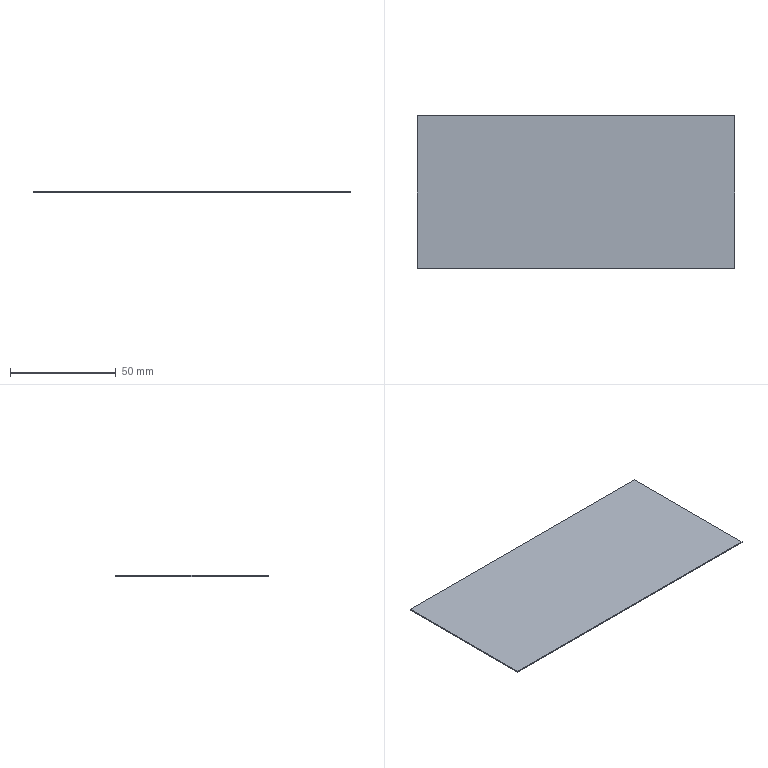Part | STEP file | Bag feed part 2 | 1 solid | 6 faces | box 150 x 72 x 0.5 mm | volume 5400 mm3 | plane 6
STEP:
#1=CARTESIAN_POINT('',(0.,0.,0.));
#2=DIRECTION('',(0.,0.,1.));
#3=DIRECTION('',(1.,0.,0.));
#4=AXIS2_PLACEMENT_3D('',#1,#2,#3);
#5=CARTESIAN_POINT('',(75.,-36.,0.));
#6=VERTEX_POINT('',#5);
#7=CARTESIAN_POINT('',(75.,36.,0.));
#8=VERTEX_POINT('',#7);
#9=CARTESIAN_POINT('',(75.,-36.,0.));
#10=DIRECTION('',(0.,1.,0.));
#11=VECTOR('',#10,1.);
#12=LINE('',#9,#11);
#13=CARTESIAN_POINT('',(75.,-36.,0.5));
#14=DIRECTION('',(-1.,0.,0.));
#15=DIRECTION('',(0.,0.,1.));
#16=AXIS2_PLACEMENT_3D('',#13,#14,#15);
#17=PLANE('',#16);
#18=CARTESIAN_POINT('',(-0.5,0.));
#19=DIRECTION('',(0.,1.));
#20=VECTOR('',#19,1.);
#21=LINE('',#18,#20);
#22=(GEOMETRIC_REPRESENTATION_CONTEXT(2)PARAMETRIC_REPRESENTATION_CONTEXT()REPRESENTATION_CONTEXT('',''));
#23=DEFINITIONAL_REPRESENTATION('',(#21),#22);
#24=PCURVE('',#17,#23);
#25=CARTESIAN_POINT('',(0.,0.,0.));
#26=DIRECTION('',(0.,0.,-1.));
#27=DIRECTION('',(-1.,0.,0.));
#28=AXIS2_PLACEMENT_3D('',#25,#26,#27);
#29=PLANE('',#28);
#30=CARTESIAN_POINT('',(-75.,-36.));
#31=DIRECTION('',(0.,1.));
#32=VECTOR('',#31,1.);
#33=LINE('',#30,#32);
#34=(GEOMETRIC_REPRESENTATION_CONTEXT(2)PARAMETRIC_REPRESENTATION_CONTEXT()REPRESENTATION_CONTEXT('',''));
#35=DEFINITIONAL_REPRESENTATION('',(#33),#34);
#36=PCURVE('',#29,#35);
#37=SURFACE_CURVE('',#12,(#24,#36),.PCURVE_S1.);
#38=EDGE_CURVE('',#6,#8,#37,.T.);
#39=ORIENTED_EDGE('',*,*,#38,.T.);
#40=CARTESIAN_POINT('',(75.,36.,0.5));
#41=VERTEX_POINT('',#40);
#42=CARTESIAN_POINT('',(75.,36.,0.5));
#43=DIRECTION('',(0.,0.,-1.));
#44=VECTOR('',#43,1.);
#45=LINE('',#42,#44);
#46=CARTESIAN_POINT('',(0.,72.));
#47=DIRECTION('',(-1.,0.));
#48=VECTOR('',#47,1.);
#49=LINE('',#46,#48);
#50=(GEOMETRIC_REPRESENTATION_CONTEXT(2)PARAMETRIC_REPRESENTATION_CONTEXT()REPRESENTATION_CONTEXT('',''));
#51=DEFINITIONAL_REPRESENTATION('',(#49),#50);
#52=PCURVE('',#17,#51);
#53=CARTESIAN_POINT('',(-75.,36.,0.5));
#54=DIRECTION('',(0.,-1.,0.));
#55=DIRECTION('',(0.,0.,-1.));
#56=AXIS2_PLACEMENT_3D('',#53,#54,#55);
#57=PLANE('',#56);
#58=CARTESIAN_POINT('',(0.,150.));
#59=DIRECTION('',(1.,0.));
#60=VECTOR('',#59,1.);
#61=LINE('',#58,#60);
#62=(GEOMETRIC_REPRESENTATION_CONTEXT(2)PARAMETRIC_REPRESENTATION_CONTEXT()REPRESENTATION_CONTEXT('',''));
#63=DEFINITIONAL_REPRESENTATION('',(#61),#62);
#64=PCURVE('',#57,#63);
#65=SURFACE_CURVE('',#45,(#52,#64),.PCURVE_S1.);
#66=EDGE_CURVE('',#41,#8,#65,.T.);
#67=ORIENTED_EDGE('',*,*,#66,.F.);
#68=CARTESIAN_POINT('',(75.,-36.,0.5));
#69=VERTEX_POINT('',#68);
#70=CARTESIAN_POINT('',(75.,-36.,0.5));
#71=DIRECTION('',(0.,1.,0.));
#72=VECTOR('',#71,1.);
#73=LINE('',#70,#72);
#74=CARTESIAN_POINT('',(0.,0.));
#75=DIRECTION('',(0.,1.));
#76=VECTOR('',#75,1.);
#77=LINE('',#74,#76);
#78=(GEOMETRIC_REPRESENTATION_CONTEXT(2)PARAMETRIC_REPRESENTATION_CONTEXT()REPRESENTATION_CONTEXT('',''));
#79=DEFINITIONAL_REPRESENTATION('',(#77),#78);
#80=PCURVE('',#17,#79);
#81=CARTESIAN_POINT('',(0.,0.,0.5));
#82=DIRECTION('',(0.,0.,-1.));
#83=DIRECTION('',(-1.,0.,0.));
#84=AXIS2_PLACEMENT_3D('',#81,#82,#83);
#85=PLANE('',#84);
#86=CARTESIAN_POINT('',(-75.,-36.));
#87=DIRECTION('',(0.,1.));
#88=VECTOR('',#87,1.);
#89=LINE('',#86,#88);
#90=(GEOMETRIC_REPRESENTATION_CONTEXT(2)PARAMETRIC_REPRESENTATION_CONTEXT()REPRESENTATION_CONTEXT('',''));
#91=DEFINITIONAL_REPRESENTATION('',(#89),#90);
#92=PCURVE('',#85,#91);
#93=SURFACE_CURVE('',#73,(#80,#92),.PCURVE_S1.);
#94=EDGE_CURVE('',#69,#41,#93,.T.);
#95=ORIENTED_EDGE('',*,*,#94,.F.);
#96=CARTESIAN_POINT('',(75.,-36.,0.5));
#97=DIRECTION('',(0.,0.,-1.));
#98=VECTOR('',#97,1.);
#99=LINE('',#96,#98);
#100=CARTESIAN_POINT('',(0.,0.));
#101=DIRECTION('',(-1.,0.));
#102=VECTOR('',#101,1.);
#103=LINE('',#100,#102);
#104=(GEOMETRIC_REPRESENTATION_CONTEXT(2)PARAMETRIC_REPRESENTATION_CONTEXT()REPRESENTATION_CONTEXT('',''));
#105=DEFINITIONAL_REPRESENTATION('',(#103),#104);
#106=PCURVE('',#17,#105);
#107=CARTESIAN_POINT('',(-75.,-36.,0.5));
#108=DIRECTION('',(0.,1.,0.));
#109=DIRECTION('',(0.,0.,1.));
#110=AXIS2_PLACEMENT_3D('',#107,#108,#109);
#111=PLANE('',#110);
#112=CARTESIAN_POINT('',(0.,150.));
#113=DIRECTION('',(-1.,0.));
#114=VECTOR('',#113,1.);
#115=LINE('',#112,#114);
#116=(GEOMETRIC_REPRESENTATION_CONTEXT(2)PARAMETRIC_REPRESENTATION_CONTEXT()REPRESENTATION_CONTEXT('',''));
#117=DEFINITIONAL_REPRESENTATION('',(#115),#116);
#118=PCURVE('',#111,#117);
#119=SURFACE_CURVE('',#99,(#106,#118),.PCURVE_S1.);
#120=EDGE_CURVE('',#69,#6,#119,.T.);
#121=ORIENTED_EDGE('',*,*,#120,.T.);
#122=EDGE_LOOP('',(#39,#67,#95,#121));
#123=FACE_BOUND('',#122,.T.);
#124=ADVANCED_FACE('',(#123),#17,.F.);
#125=CARTESIAN_POINT('',(-75.,36.,0.));
#126=VERTEX_POINT('',#125);
#127=CARTESIAN_POINT('',(-75.,36.,0.));
#128=DIRECTION('',(-1.,0.,0.));
#129=VECTOR('',#128,1.);
#130=LINE('',#127,#129);
#131=CARTESIAN_POINT('',(0.5,0.));
#132=DIRECTION('',(0.,-1.));
#133=VECTOR('',#132,1.);
#134=LINE('',#131,#133);
#135=(GEOMETRIC_REPRESENTATION_CONTEXT(2)PARAMETRIC_REPRESENTATION_CONTEXT()REPRESENTATION_CONTEXT('',''));
#136=DEFINITIONAL_REPRESENTATION('',(#134),#135);
#137=PCURVE('',#57,#136);
#138=CARTESIAN_POINT('',(75.,36.));
#139=DIRECTION('',(1.,0.));
#140=VECTOR('',#139,1.);
#141=LINE('',#138,#140);
#142=(GEOMETRIC_REPRESENTATION_CONTEXT(2)PARAMETRIC_REPRESENTATION_CONTEXT()REPRESENTATION_CONTEXT('',''));
#143=DEFINITIONAL_REPRESENTATION('',(#141),#142);
#144=PCURVE('',#29,#143);
#145=SURFACE_CURVE('',#130,(#137,#144),.PCURVE_S1.);
#146=EDGE_CURVE('',#8,#126,#145,.T.);
#147=ORIENTED_EDGE('',*,*,#146,.T.);
#148=CARTESIAN_POINT('',(-75.,36.,0.5));
#149=VERTEX_POINT('',#148);
#150=CARTESIAN_POINT('',(-75.,36.,0.5));
#151=DIRECTION('',(0.,0.,-1.));
#152=VECTOR('',#151,1.);
#153=LINE('',#150,#152);
#154=CARTESIAN_POINT('',(0.,0.));
#155=DIRECTION('',(1.,0.));
#156=VECTOR('',#155,1.);
#157=LINE('',#154,#156);
#158=(GEOMETRIC_REPRESENTATION_CONTEXT(2)PARAMETRIC_REPRESENTATION_CONTEXT()REPRESENTATION_CONTEXT('',''));
#159=DEFINITIONAL_REPRESENTATION('',(#157),#158);
#160=PCURVE('',#57,#159);
#161=CARTESIAN_POINT('',(-75.,-36.,0.5));
#162=DIRECTION('',(1.,0.,0.));
#163=DIRECTION('',(0.,0.,-1.));
#164=AXIS2_PLACEMENT_3D('',#161,#162,#163);
#165=PLANE('',#164);
#166=CARTESIAN_POINT('',(0.,72.));
#167=DIRECTION('',(1.,0.));
#168=VECTOR('',#167,1.);
#169=LINE('',#166,#168);
#170=(GEOMETRIC_REPRESENTATION_CONTEXT(2)PARAMETRIC_REPRESENTATION_CONTEXT()REPRESENTATION_CONTEXT('',''));
#171=DEFINITIONAL_REPRESENTATION('',(#169),#170);
#172=PCURVE('',#165,#171);
#173=SURFACE_CURVE('',#153,(#160,#172),.PCURVE_S1.);
#174=EDGE_CURVE('',#149,#126,#173,.T.);
#175=ORIENTED_EDGE('',*,*,#174,.F.);
#176=CARTESIAN_POINT('',(-75.,36.,0.5));
#177=DIRECTION('',(-1.,0.,0.));
#178=VECTOR('',#177,1.);
#179=LINE('',#176,#178);
#180=CARTESIAN_POINT('',(0.,0.));
#181=DIRECTION('',(0.,-1.));
#182=VECTOR('',#181,1.);
#183=LINE('',#180,#182);
#184=(GEOMETRIC_REPRESENTATION_CONTEXT(2)PARAMETRIC_REPRESENTATION_CONTEXT()REPRESENTATION_CONTEXT('',''));
#185=DEFINITIONAL_REPRESENTATION('',(#183),#184);
#186=PCURVE('',#57,#185);
#187=CARTESIAN_POINT('',(75.,36.));
#188=DIRECTION('',(1.,0.));
#189=VECTOR('',#188,1.);
#190=LINE('',#187,#189);
#191=(GEOMETRIC_REPRESENTATION_CONTEXT(2)PARAMETRIC_REPRESENTATION_CONTEXT()REPRESENTATION_CONTEXT('',''));
#192=DEFINITIONAL_REPRESENTATION('',(#190),#191);
#193=PCURVE('',#85,#192);
#194=SURFACE_CURVE('',#179,(#186,#193),.PCURVE_S1.);
#195=EDGE_CURVE('',#41,#149,#194,.T.);
#196=ORIENTED_EDGE('',*,*,#195,.F.);
#197=ORIENTED_EDGE('',*,*,#66,.T.);
#198=EDGE_LOOP('',(#147,#175,#196,#197));
#199=FACE_BOUND('',#198,.T.);
#200=ADVANCED_FACE('',(#199),#57,.F.);
#201=CARTESIAN_POINT('',(-75.,-36.,0.));
#202=VERTEX_POINT('',#201);
#203=CARTESIAN_POINT('',(-75.,-36.,0.));
#204=DIRECTION('',(0.,-1.,0.));
#205=VECTOR('',#204,1.);
#206=LINE('',#203,#205);
#207=CARTESIAN_POINT('',(0.5,0.));
#208=DIRECTION('',(0.,-1.));
#209=VECTOR('',#208,1.);
#210=LINE('',#207,#209);
#211=(GEOMETRIC_REPRESENTATION_CONTEXT(2)PARAMETRIC_REPRESENTATION_CONTEXT()REPRESENTATION_CONTEXT('',''));
#212=DEFINITIONAL_REPRESENTATION('',(#210),#211);
#213=PCURVE('',#165,#212);
#214=CARTESIAN_POINT('',(75.,-36.));
#215=DIRECTION('',(0.,-1.));
#216=VECTOR('',#215,1.);
#217=LINE('',#214,#216);
#218=(GEOMETRIC_REPRESENTATION_CONTEXT(2)PARAMETRIC_REPRESENTATION_CONTEXT()REPRESENTATION_CONTEXT('',''));
#219=DEFINITIONAL_REPRESENTATION('',(#217),#218);
#220=PCURVE('',#29,#219);
#221=SURFACE_CURVE('',#206,(#213,#220),.PCURVE_S1.);
#222=EDGE_CURVE('',#126,#202,#221,.T.);
#223=ORIENTED_EDGE('',*,*,#222,.T.);
#224=CARTESIAN_POINT('',(-75.,-36.,0.5));
#225=VERTEX_POINT('',#224);
#226=CARTESIAN_POINT('',(-75.,-36.,0.5));
#227=DIRECTION('',(0.,0.,-1.));
#228=VECTOR('',#227,1.);
#229=LINE('',#226,#228);
#230=CARTESIAN_POINT('',(0.,0.));
#231=DIRECTION('',(1.,0.));
#232=VECTOR('',#231,1.);
#233=LINE('',#230,#232);
#234=(GEOMETRIC_REPRESENTATION_CONTEXT(2)PARAMETRIC_REPRESENTATION_CONTEXT()REPRESENTATION_CONTEXT('',''));
#235=DEFINITIONAL_REPRESENTATION('',(#233),#234);
#236=PCURVE('',#165,#235);
#237=CARTESIAN_POINT('',(0.,0.));
#238=DIRECTION('',(-1.,0.));
#239=VECTOR('',#238,1.);
#240=LINE('',#237,#239);
#241=(GEOMETRIC_REPRESENTATION_CONTEXT(2)PARAMETRIC_REPRESENTATION_CONTEXT()REPRESENTATION_CONTEXT('',''));
#242=DEFINITIONAL_REPRESENTATION('',(#240),#241);
#243=PCURVE('',#111,#242);
#244=SURFACE_CURVE('',#229,(#236,#243),.PCURVE_S1.);
#245=EDGE_CURVE('',#225,#202,#244,.T.);
#246=ORIENTED_EDGE('',*,*,#245,.F.);
#247=CARTESIAN_POINT('',(-75.,-36.,0.5));
#248=DIRECTION('',(0.,-1.,0.));
#249=VECTOR('',#248,1.);
#250=LINE('',#247,#249);
#251=CARTESIAN_POINT('',(0.,0.));
#252=DIRECTION('',(0.,-1.));
#253=VECTOR('',#252,1.);
#254=LINE('',#251,#253);
#255=(GEOMETRIC_REPRESENTATION_CONTEXT(2)PARAMETRIC_REPRESENTATION_CONTEXT()REPRESENTATION_CONTEXT('',''));
#256=DEFINITIONAL_REPRESENTATION('',(#254),#255);
#257=PCURVE('',#165,#256);
#258=CARTESIAN_POINT('',(75.,-36.));
#259=DIRECTION('',(0.,-1.));
#260=VECTOR('',#259,1.);
#261=LINE('',#258,#260);
#262=(GEOMETRIC_REPRESENTATION_CONTEXT(2)PARAMETRIC_REPRESENTATION_CONTEXT()REPRESENTATION_CONTEXT('',''));
#263=DEFINITIONAL_REPRESENTATION('',(#261),#262);
#264=PCURVE('',#85,#263);
#265=SURFACE_CURVE('',#250,(#257,#264),.PCURVE_S1.);
#266=EDGE_CURVE('',#149,#225,#265,.T.);
#267=ORIENTED_EDGE('',*,*,#266,.F.);
#268=ORIENTED_EDGE('',*,*,#174,.T.);
#269=EDGE_LOOP('',(#223,#246,#267,#268));
#270=FACE_BOUND('',#269,.T.);
#271=ADVANCED_FACE('',(#270),#165,.F.);
#272=CARTESIAN_POINT('',(-75.,-36.,0.));
#273=DIRECTION('',(1.,0.,0.));
#274=VECTOR('',#273,1.);
#275=LINE('',#272,#274);
#276=CARTESIAN_POINT('',(-0.5,0.));
#277=DIRECTION('',(0.,1.));
#278=VECTOR('',#277,1.);
#279=LINE('',#276,#278);
#280=(GEOMETRIC_REPRESENTATION_CONTEXT(2)PARAMETRIC_REPRESENTATION_CONTEXT()REPRESENTATION_CONTEXT('',''));
#281=DEFINITIONAL_REPRESENTATION('',(#279),#280);
#282=PCURVE('',#111,#281);
#283=CARTESIAN_POINT('',(75.,-36.));
#284=DIRECTION('',(-1.,0.));
#285=VECTOR('',#284,1.);
#286=LINE('',#283,#285);
#287=(GEOMETRIC_REPRESENTATION_CONTEXT(2)PARAMETRIC_REPRESENTATION_CONTEXT()REPRESENTATION_CONTEXT('',''));
#288=DEFINITIONAL_REPRESENTATION('',(#286),#287);
#289=PCURVE('',#29,#288);
#290=SURFACE_CURVE('',#275,(#282,#289),.PCURVE_S1.);
#291=EDGE_CURVE('',#202,#6,#290,.T.);
#292=ORIENTED_EDGE('',*,*,#291,.T.);
#293=ORIENTED_EDGE('',*,*,#120,.F.);
#294=CARTESIAN_POINT('',(-75.,-36.,0.5));
#295=DIRECTION('',(1.,0.,0.));
#296=VECTOR('',#295,1.);
#297=LINE('',#294,#296);
#298=CARTESIAN_POINT('',(0.,0.));
#299=DIRECTION('',(0.,1.));
#300=VECTOR('',#299,1.);
#301=LINE('',#298,#300);
#302=(GEOMETRIC_REPRESENTATION_CONTEXT(2)PARAMETRIC_REPRESENTATION_CONTEXT()REPRESENTATION_CONTEXT('',''));
#303=DEFINITIONAL_REPRESENTATION('',(#301),#302);
#304=PCURVE('',#111,#303);
#305=CARTESIAN_POINT('',(75.,-36.));
#306=DIRECTION('',(-1.,0.));
#307=VECTOR('',#306,1.);
#308=LINE('',#305,#307);
#309=(GEOMETRIC_REPRESENTATION_CONTEXT(2)PARAMETRIC_REPRESENTATION_CONTEXT()REPRESENTATION_CONTEXT('',''));
#310=DEFINITIONAL_REPRESENTATION('',(#308),#309);
#311=PCURVE('',#85,#310);
#312=SURFACE_CURVE('',#297,(#304,#311),.PCURVE_S1.);
#313=EDGE_CURVE('',#225,#69,#312,.T.);
#314=ORIENTED_EDGE('',*,*,#313,.F.);
#315=ORIENTED_EDGE('',*,*,#245,.T.);
#316=EDGE_LOOP('',(#292,#293,#314,#315));
#317=FACE_BOUND('',#316,.T.);
#318=ADVANCED_FACE('',(#317),#111,.F.);
#319=ORIENTED_EDGE('',*,*,#94,.T.);
#320=ORIENTED_EDGE('',*,*,#195,.T.);
#321=ORIENTED_EDGE('',*,*,#266,.T.);
#322=ORIENTED_EDGE('',*,*,#313,.T.);
#323=EDGE_LOOP('',(#319,#320,#321,#322));
#324=FACE_BOUND('',#323,.T.);
#325=ADVANCED_FACE('',(#324),#85,.F.);
#326=ORIENTED_EDGE('',*,*,#38,.F.);
#327=ORIENTED_EDGE('',*,*,#291,.F.);
#328=ORIENTED_EDGE('',*,*,#222,.F.);
#329=ORIENTED_EDGE('',*,*,#146,.F.);
#330=EDGE_LOOP('',(#326,#327,#328,#329));
#331=FACE_BOUND('',#330,.T.);
#332=ADVANCED_FACE('',(#331),#29,.T.);
#333=CLOSED_SHELL('',(#124,#200,#271,#318,#325,#332));
#334=MANIFOLD_SOLID_BREP('',#333);
#335=(LENGTH_UNIT()NAMED_UNIT(*)SI_UNIT(.MILLI.,.METRE.));
#336=UNCERTAINTY_MEASURE_WITH_UNIT(LENGTH_MEASURE(0.0000001),#335,'','');
#337=(NAMED_UNIT(*)PLANE_ANGLE_UNIT()SI_UNIT($,.RADIAN.));
#338=(NAMED_UNIT(*)SI_UNIT($,.STERADIAN.)SOLID_ANGLE_UNIT());
#339=(GEOMETRIC_REPRESENTATION_CONTEXT(3)GLOBAL_UNCERTAINTY_ASSIGNED_CONTEXT((#336))GLOBAL_UNIT_ASSIGNED_CONTEXT((#335,#337,#338))REPRESENTATION_CONTEXT('',''));
#340=ADVANCED_BREP_SHAPE_REPRESENTATION('',(#4,#334),#339);